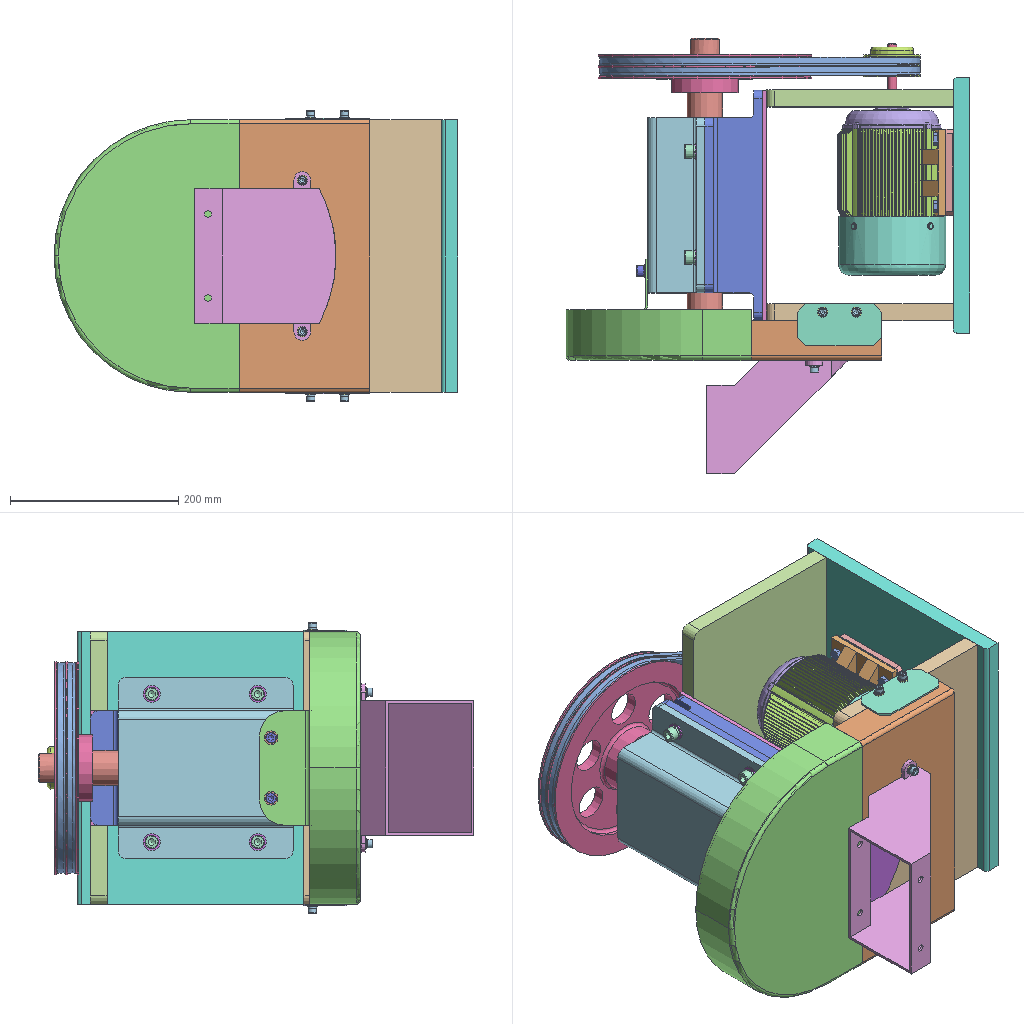Assembly | NX | 30 different items | 61 placed | box 480 x 518 x 346 mm
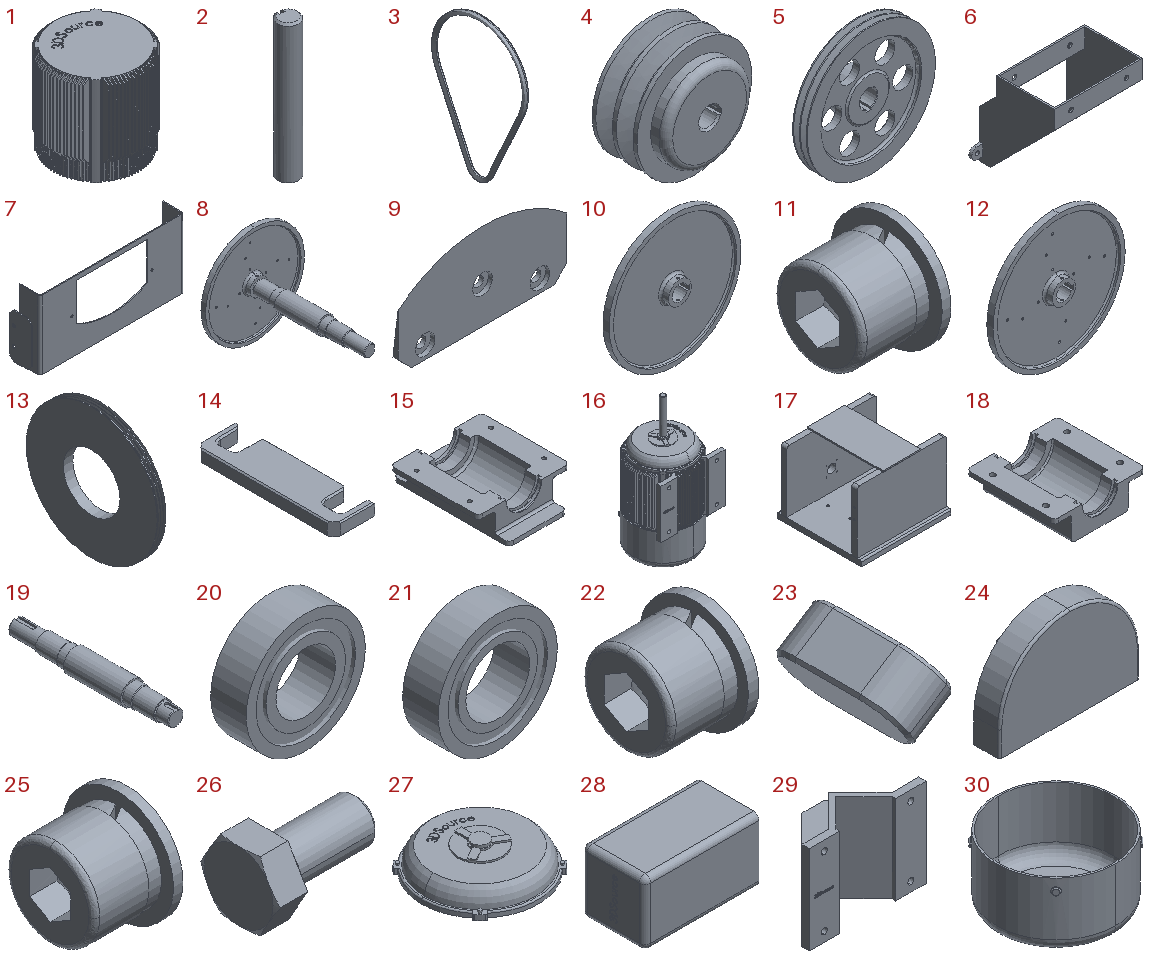Parts list (item | quantity | parent item | size | volume | features):
1 | x1 | in 16 | 130 x 130 x 127.333 mm | 1463982 mm3 | features BREP 1
2 | x1 | in 16 | 11 x 12 x 73 mm | 6944 mm3 | features DATUM_CSYS 3, EXTRUDE 3, SKETCH 3, BLEND 2, BREP 1, CHAMFER 1
3 | x2 | - | 10.196 x 249.988 x 380.986 mm | 61835 mm3 | features DATUM_CSYS 2, SKETCH 2, DATUM_ON_PATH 1, SKIN 1
4 | x1 | - | 67 x 35 x 67 mm | 82909 mm3 | features DATUM_CSYS 3, SKETCH 2, BLEND 1, CHAMFER 1, EXTRUDE 1, SWP104 1
5 | x1 | - | 254 x 45.355 x 254 mm | 836856 mm3 | features DATUM_CSYS 9, SKETCH 8, EXTRACT_DATUM_AXIS 6, EXTRACT_FACE 6, HOLE PACKAGE 6, SIMPLE HOLE 6, Instance Feature 5, BLEND 2, EXTRUDE 1, Pattern Feature 1, SWP104 1
6 | x1 | - | 200 x 135 x 168 mm | 211668 mm3 | features DATUM_CSYS 6, SKETCH 5, EXTRUDE 4, HOLE PACKAGE 4, SIMPLE HOLE 4, BLEND 2, EXTRACT_FACE 2, EXTRACT_STRING 2, DATUM_PLANE 1, Instance Feature 1, Mirror Feature 1, SHELL 1
7 | x1 | - | 328 x 67 x 155 mm | 114572 mm3 | features BREP 3
8 | x1 | - | 300 x 374.3 x 300 mm | 1215176 mm3 | features DATUM_CSYS 10, SKETCH 8, EXTRUDE 5, BREP 4, EXTRACT_DATUM_AXIS 3, EXTRACT_DATUM_PLANE 3, EXTRACT_FACE 3, EXTRACT_STRING 3, HOLE PACKAGE 3, SIMPLE HOLE 3, CHAMFER 2, Instance Feature 2, SWP104 2, BLEND 1, DATUM_PLANE 1, Pattern Feature 1
9 | x4 | in 8 | 103 x 5 x 53 mm | 14704 mm3 | features DATUM_CSYS 7, SKETCH 6, EXTRUDE 4, EXTRACT_DATUM_AXIS 3, EXTRACT_DATUM_PLANE 3, EXTRACT_FACE 3, EXTRACT_STRING 3, HOLE PACKAGE 3, SIMPLE HOLE 3, Instance Feature 2, CHAMFER 1, Pattern Feature 1, SWP104 1
10 | x1 | - | 300 x 25 x 300 mm | 574128 mm3 | features DATUM_CSYS 5, SKETCH 4, EXTRUDE 3, BLEND 2, DATUM_PLANE 1, SWP104 1
11 | x4 | - | 14.1 x 20.25 x 20.25 mm | 2295 mm3 | features BREP 2
12 | x1 | in 8 | 300 x 25 x 300 mm | 572533 mm3 | features BREP 1
13 | x2 | - | 7 x 97 x 97 mm | 39442 mm3 | features DATUM_CSYS 3, SKETCH 2, CHAMFER 1, EXTRUDE 1, SWP104 1
14 | x2 | - | 30 x 102.4 x 9.5 mm | 22943 mm3 | features CHAMFER 3, DATUM_CSYS 3, EXTRUDE 3, BLEND 2, EXTRACT_STRING 2, SKETCH 2, Instance Feature 1, Pattern Feature 1
15 | x1 | - | 216 x 274 x 68 mm | 1265227 mm3 | features DATUM_CSYS 8, SKETCH 7, EXTRACT_FACE 4, HOLE PACKAGE 4, SIMPLE HOLE 4, SYMBOLIC_THREAD 4, Instance Feature 3, BLEND 2, EXTRUDE 2, CHAMFER 1, DATUM_PLANE 1, Pattern Feature 1, SWP104 1, UNITE 1
16 | x1 | - | 137.5 x 130 x 275 mm | 2091891 mm3 | features BREP 6, DATUM_CSYS 3, EXTRUDE 3, SKETCH 3, BLEND 2, CHAMFER 1
17 | x1 | - | 324 x 304 x 247 mm | 5008657 mm3 | features DATUM_CSYS 14, SKETCH 13, EXTRACT_FACE 10, HOLE PACKAGE 8, SIMPLE HOLE 8, SYMBOLIC_THREAD 8, Instance Feature 6, EXTRACT_STRING 5, EXTRUDE 5, Pattern Feature 3, BLEND 2, CHAMFER 1, Mirror Feature 1, Pattern Geometry 1
18 | x1 | - | 216 x 208 x 68 mm | 1158668 mm3 | features DATUM_CSYS 10, SKETCH 9, EXTRACT_FACE 6, HOLE PACKAGE 6, SIMPLE HOLE 6, BLEND 4, Instance Feature 4, EXTRUDE 2, Pattern Feature 2, SYMBOLIC_THREAD 2, CHAMFER 1, DATUM_PLANE 1, SWP104 1
19 | x1 | in 8 | 53 x 363 x 53 mm | 574308 mm3 | features DATUM_CSYS 3, SKETCH 2, BLEND 1, CHAMFER 1, DATUM_PLANE 1, EXTRUDE 1, SWP104 1
20 | x1 | - | 84 x 25 x 84 mm | 100939 mm3 | features DATUM_CSYS 4, EXTRUDE 3, SKETCH 3
21 | x1 | - | 84 x 25 x 84 mm | 95815 mm3 | features DATUM_CSYS 4, EXTRUDE 3, SKETCH 3
22 | x18 | in 8 | 8.8 x 12.2 x 12.2 mm | 563.29 mm3 | features BREP 2
23 | x2 | in 8 | 11.452 x 20 x 12.091 mm | 1380 mm3 | features BREP 1
24 | x1 | - | 324 x 120 x 220 mm | 283297 mm3 | features BREP 1
25 | x2 | - | 11.4 x 16.2 x 16.2 mm | 1258 mm3 | features BREP 2
26 | x4 | - | 21.95 x 14.699 x 12.73 mm | 1621 mm3 | features BREP 1
27 | x1 | in 16 | 117 x 117 x 28 mm | 208351 mm3 | features BREP 1
28 | x1 | in 16 | 70 x 39 x 39 mm | 105347 mm3 | features BREP 1
29 | x1 | in 16 | 135 x 63 x 102.4 mm | 230234 mm3 | features BREP 1
30 | x1 | in 16 | 127.4 x 127.4 x 70 mm | 77039 mm3 | features BREP 1
Mates (type | each side: item.copy, entity, surface, feature):
In the top assembly
Touch | 19.1 face cylinder Revolve(2) | 15.1 face cylinder Revolve(8)
Touch | 19.1 face plane Revolve(2) | 15.1 face plane Revolve(8)
Touch | 18.1 face plane Extrude(4) | 15.1 face plane Extrude(4)
Touch | 18.1 face cylinder Pattern Feature [Linear] (9) / Instance[1][0] | 15.1 face cylinder Pattern Feature [Linear] (13) / Instance[1][1]
Touch | 5.1 face cylinder Revolve(2) | 19.1 face cylinder Revolve(2)
Touch | 5.1 face plane Revolve(2) | 19.1 face plane Revolve(2)
Parallel | 5.1 face plane Extrude(6) | 19.1 face plane Extrude(7)
Distance | 7.1 face plane Body(1) | 17.1 face plane Extrude(2)
Touch | 7.1 face plane Body(1) | 17.1 face plane Pattern Feature [Linear] (5) / Instance[1][0]
Touch | 24.1 face plane Body(1) | 7.1 face plane Body(1) | 3 times
Touch | 7.1 face plane Body(3) | 17.1 face plane Pattern Feature [Linear] (5) / Instance[1][0]
Distance | 18.1 face plane Extrude(2) | 17.1 face plane Extrude(4)
Touch | 6.1 face cylinder Mirror Feature(9) | 7.1 face cylinder Body(1) | 2 times
Touch | 6.1 face cylinder Ø7 Hole(7) | 7.1 face cylinder Body(1) | 2 times
Touch | 6.1 face plane Extrude(2) | 7.1 face plane Body(1)
Touch | 15.1 face plane Extrude(2) | 17.1 face plane Extrude(4)
Touch | 15.1 face plane Extrude(2) | 17.1 face plane Extrude(7) | 2 times
Touch | 4.1 face plane Revolve(2) | 5.1 face plane Revolve(2)
Touch | 3.1 | 4.1 face cylinder Revolve(2) | 2 times
Touch | 3.1 | 19.1 face cylinder Revolve(2)
Touch | 3.1 | 5.1 face cylinder Revolve(2)
Touch | 20.1 face cylinder Extrude(2) | 19.1 face cylinder Revolve(2)
Touch | 20.1 face plane Extrude(4) | 19.1 face plane Revolve(2)
Touch | 21.1 face cylinder Extrude(4) | 15.1 face cylinder Revolve(8)
Touch | 21.1 face plane Extrude(2) | 19.1 face plane Revolve(2)
Touch | 13.1 face cylinder Extrude(2) | 19.1 face cylinder Revolve(2) | 2 times
Touch | 13.1 face plane Extrude(2) | 15.1 face plane Revolve(8) | 2 times
Concentric | 25.1 edge | 24.1 edge | 2 times
Concentric | 11.1 edge | 18.1 edge | 4 times
Concentric | 17.1 edge | 7.1 edge
Concentric | 7.1 edge | 17.1 edge
Concentric | 22.1 edge | 7.1 edge | 4 times
Concentric | 22.1 edge | 6.1 edge | 2 times
Parallel | 29.1 face plane Body(1) | 17.1 face plane Extrude(2)
Concentric | 26.1 edge | 29.1 edge | 4 times
Distance | 30.1 face plane Body(1) | 17.1 face plane Extrude(4)
Touch | 26.1 face cylinder Body(1) | 17.1 face cylinder M8 x 1.25 Threaded Hole(20)
Touch | 26.1 face cylinder Body(1) | 17.1 face cylinder Pattern Feature [Linear] (21) / Instance[1][0]
Touch | 14.1 face plane Extrude(2) | 17.1 face plane Extrude(2) | 2 times
Touch | 14.1 face plane Extrude(2) | 29.1 face plane Body(1) | 4 times
Touch | 4.1 face cylinder Revolve(2) | 2.1 face cylinder Body(0)
In subassembly 8
Parallel | 19.1 | 12.1
Touch | 12.1 | 19.1
Touch | 19.1 | 12.1
Concentric | 9.1 | 12.1 | 6 times
Concentric | 12.1 | 9.1 | 3 times
Touch | 23.1 face plane Body(1) | 19.1 | 4 times
Touch | 23.1 face cylinder Body(1) | 19.1 | 2 times
Concentric | 22.1 edge | 9.1
Concentric | 22.1 | 9.1 | 11 times
In subassembly 16
Concentric | 2.1 | 27.1
Fix | 29.1 component
Touch | 2.1 | 1.1